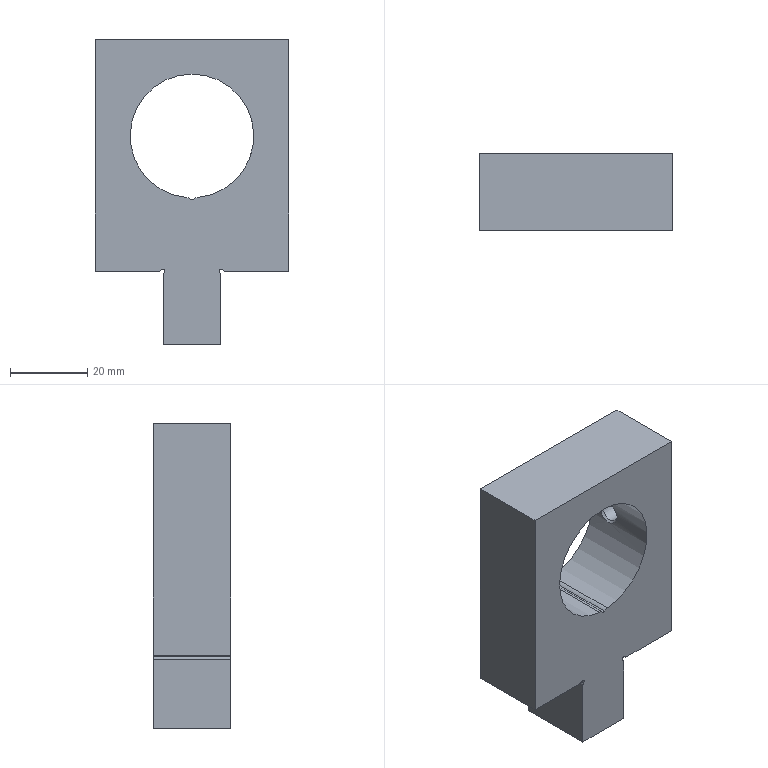Part | STEP file | YBQDJ-DX-BD-2 | 1 solid | 23 faces | box 50 x 20 x 79 mm | volume 49384 mm3 | cylinder 11 | plane 10 | cone 1 | spline 1 | commonest cylinder face diameters 2 x4 1 x3 4 x2 5 x1 32.01 x1